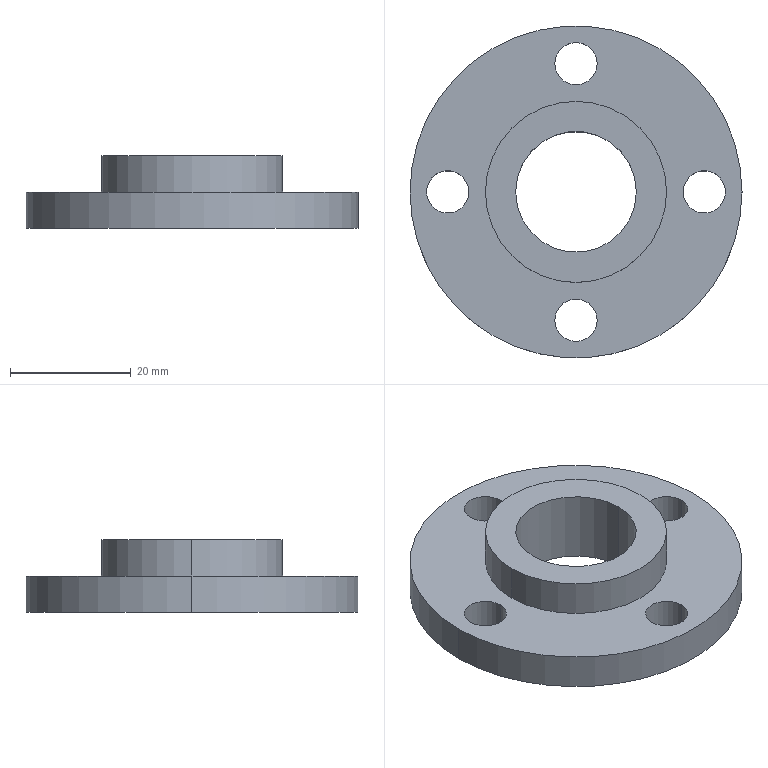Part | STEP file | BCC3 H16_9 | 1 solid | 17 faces | box 55 x 55 x 12 mm | volume 13803 mm3 | cylinder 14 | plane 3 | commonest cylinder face diameters 7 x8 20 x2 30 x2 55 x2
STEP:
#1=CARTESIAN_POINT('',(0.,0.,0.));
#2=DIRECTION('',(0.,0.,1.));
#3=DIRECTION('',(1.,0.,0.));
#4=AXIS2_PLACEMENT_3D('',#1,#2,#3);
#5=CARTESIAN_POINT('',(-17.75,0.,0.));
#6=VERTEX_POINT('',#5);
#7=CARTESIAN_POINT('',(-17.75,0.,6.));
#8=VERTEX_POINT('',#7);
#9=CARTESIAN_POINT('',(-17.75,0.,0.));
#10=DIRECTION('',(0.,0.,1.));
#11=VECTOR('',#10,1.);
#12=LINE('',#9,#11);
#13=CARTESIAN_POINT('',(-21.25,0.,0.));
#14=DIRECTION('',(0.,0.,1.));
#15=DIRECTION('',(1.,0.,0.));
#16=AXIS2_PLACEMENT_3D('',#13,#14,#15);
#17=CYLINDRICAL_SURFACE('',#16,3.5);
#18=CARTESIAN_POINT('',(6.283,0.));
#19=DIRECTION('',(0.,1.));
#20=VECTOR('',#19,1.);
#21=LINE('',#18,#20);
#22=(GEOMETRIC_REPRESENTATION_CONTEXT(2)PARAMETRIC_REPRESENTATION_CONTEXT()REPRESENTATION_CONTEXT('',''));
#23=DEFINITIONAL_REPRESENTATION('',(#21),#22);
#24=PCURVE('',#17,#23);
#25=CARTESIAN_POINT('',(-21.25,0.,0.));
#26=DIRECTION('',(0.,0.,1.));
#27=DIRECTION('',(1.,0.,0.));
#28=AXIS2_PLACEMENT_3D('',#25,#26,#27);
#29=CYLINDRICAL_SURFACE('',#28,3.5);
#30=CARTESIAN_POINT('',(0.,0.));
#31=DIRECTION('',(0.,1.));
#32=VECTOR('',#31,1.);
#33=LINE('',#30,#32);
#34=(GEOMETRIC_REPRESENTATION_CONTEXT(2)PARAMETRIC_REPRESENTATION_CONTEXT()REPRESENTATION_CONTEXT('',''));
#35=DEFINITIONAL_REPRESENTATION('',(#33),#34);
#36=PCURVE('',#29,#35);
#37=SURFACE_CURVE('',#12,(#24,#36),.PCURVE_S1.);
#38=EDGE_CURVE('',#6,#8,#37,.T.);
#39=ORIENTED_EDGE('',*,*,#38,.T.);
#40=CARTESIAN_POINT('',(-24.75,0.,6.));
#41=VERTEX_POINT('',#40);
#42=CARTESIAN_POINT('',(-21.25,0.,6.));
#43=DIRECTION('',(0.,0.,1.));
#44=DIRECTION('',(0.,1.,0.));
#45=AXIS2_PLACEMENT_3D('',#42,#43,#44);
#46=CIRCLE('',#45,3.5);
#47=CARTESIAN_POINT('',(1.571,6.));
#48=DIRECTION('',(1.,0.));
#49=VECTOR('',#48,1.);
#50=LINE('',#47,#49);
#51=(GEOMETRIC_REPRESENTATION_CONTEXT(2)PARAMETRIC_REPRESENTATION_CONTEXT()REPRESENTATION_CONTEXT('',''));
#52=DEFINITIONAL_REPRESENTATION('',(#50),#51);
#53=PCURVE('',#17,#52);
#54=CARTESIAN_POINT('',(0.,0.,6.));
#55=DIRECTION('',(0.,0.,1.));
#56=DIRECTION('',(1.,0.,0.));
#57=AXIS2_PLACEMENT_3D('',#54,#55,#56);
#58=PLANE('',#57);
#59=CARTESIAN_POINT('',(-21.25,0.));
#60=DIRECTION('',(0.,1.));
#61=AXIS2_PLACEMENT_2D('',#59,#60);
#62=CIRCLE('',#61,3.5);
#63=(GEOMETRIC_REPRESENTATION_CONTEXT(2)PARAMETRIC_REPRESENTATION_CONTEXT()REPRESENTATION_CONTEXT('',''));
#64=DEFINITIONAL_REPRESENTATION('',(#62),#63);
#65=PCURVE('',#58,#64);
#66=SURFACE_CURVE('',#46,(#53,#65),.PCURVE_S1.);
#67=EDGE_CURVE('',#41,#8,#66,.T.);
#68=ORIENTED_EDGE('',*,*,#67,.F.);
#69=CARTESIAN_POINT('',(-24.75,0.,0.));
#70=VERTEX_POINT('',#69);
#71=CARTESIAN_POINT('',(-24.75,0.,0.));
#72=DIRECTION('',(0.,0.,1.));
#73=VECTOR('',#72,1.);
#74=LINE('',#71,#73);
#75=CARTESIAN_POINT('',(3.142,0.));
#76=DIRECTION('',(0.,1.));
#77=VECTOR('',#76,1.);
#78=LINE('',#75,#77);
#79=(GEOMETRIC_REPRESENTATION_CONTEXT(2)PARAMETRIC_REPRESENTATION_CONTEXT()REPRESENTATION_CONTEXT('',''));
#80=DEFINITIONAL_REPRESENTATION('',(#78),#79);
#81=PCURVE('',#17,#80);
#82=CARTESIAN_POINT('',(3.142,0.));
#83=DIRECTION('',(0.,1.));
#84=VECTOR('',#83,1.);
#85=LINE('',#82,#84);
#86=(GEOMETRIC_REPRESENTATION_CONTEXT(2)PARAMETRIC_REPRESENTATION_CONTEXT()REPRESENTATION_CONTEXT('',''));
#87=DEFINITIONAL_REPRESENTATION('',(#85),#86);
#88=PCURVE('',#29,#87);
#89=SURFACE_CURVE('',#74,(#81,#88),.PCURVE_S1.);
#90=EDGE_CURVE('',#70,#41,#89,.T.);
#91=ORIENTED_EDGE('',*,*,#90,.F.);
#92=CARTESIAN_POINT('',(-21.25,0.,0.));
#93=DIRECTION('',(0.,0.,1.));
#94=DIRECTION('',(0.,1.,0.));
#95=AXIS2_PLACEMENT_3D('',#92,#93,#94);
#96=CIRCLE('',#95,3.5);
#97=CARTESIAN_POINT('',(1.571,0.));
#98=DIRECTION('',(1.,0.));
#99=VECTOR('',#98,1.);
#100=LINE('',#97,#99);
#101=(GEOMETRIC_REPRESENTATION_CONTEXT(2)PARAMETRIC_REPRESENTATION_CONTEXT()REPRESENTATION_CONTEXT('',''));
#102=DEFINITIONAL_REPRESENTATION('',(#100),#101);
#103=PCURVE('',#17,#102);
#104=CARTESIAN_POINT('',(0.,0.,0.));
#105=DIRECTION('',(0.,0.,1.));
#106=DIRECTION('',(1.,0.,0.));
#107=AXIS2_PLACEMENT_3D('',#104,#105,#106);
#108=PLANE('',#107);
#109=CARTESIAN_POINT('',(-21.25,0.));
#110=DIRECTION('',(0.,1.));
#111=AXIS2_PLACEMENT_2D('',#109,#110);
#112=CIRCLE('',#111,3.5);
#113=(GEOMETRIC_REPRESENTATION_CONTEXT(2)PARAMETRIC_REPRESENTATION_CONTEXT()REPRESENTATION_CONTEXT('',''));
#114=DEFINITIONAL_REPRESENTATION('',(#112),#113);
#115=PCURVE('',#108,#114);
#116=SURFACE_CURVE('',#96,(#103,#115),.PCURVE_S1.);
#117=EDGE_CURVE('',#70,#6,#116,.T.);
#118=ORIENTED_EDGE('',*,*,#117,.T.);
#119=EDGE_LOOP('',(#39,#68,#91,#118));
#120=FACE_BOUND('',#119,.F.);
#121=ADVANCED_FACE('',(#120),#17,.F.);
#122=CARTESIAN_POINT('',(3.5,-21.25,0.));
#123=VERTEX_POINT('',#122);
#124=CARTESIAN_POINT('',(3.5,-21.25,6.));
#125=VERTEX_POINT('',#124);
#126=CARTESIAN_POINT('',(3.5,-21.25,0.));
#127=DIRECTION('',(0.,0.,1.));
#128=VECTOR('',#127,1.);
#129=LINE('',#126,#128);
#130=CARTESIAN_POINT('',(0.,-21.25,0.));
#131=DIRECTION('',(0.,0.,1.));
#132=DIRECTION('',(1.,0.,0.));
#133=AXIS2_PLACEMENT_3D('',#130,#131,#132);
#134=CYLINDRICAL_SURFACE('',#133,3.5);
#135=CARTESIAN_POINT('',(6.283,0.));
#136=DIRECTION('',(0.,1.));
#137=VECTOR('',#136,1.);
#138=LINE('',#135,#137);
#139=(GEOMETRIC_REPRESENTATION_CONTEXT(2)PARAMETRIC_REPRESENTATION_CONTEXT()REPRESENTATION_CONTEXT('',''));
#140=DEFINITIONAL_REPRESENTATION('',(#138),#139);
#141=PCURVE('',#134,#140);
#142=CARTESIAN_POINT('',(0.,-21.25,0.));
#143=DIRECTION('',(0.,0.,1.));
#144=DIRECTION('',(1.,0.,0.));
#145=AXIS2_PLACEMENT_3D('',#142,#143,#144);
#146=CYLINDRICAL_SURFACE('',#145,3.5);
#147=CARTESIAN_POINT('',(0.,0.));
#148=DIRECTION('',(0.,1.));
#149=VECTOR('',#148,1.);
#150=LINE('',#147,#149);
#151=(GEOMETRIC_REPRESENTATION_CONTEXT(2)PARAMETRIC_REPRESENTATION_CONTEXT()REPRESENTATION_CONTEXT('',''));
#152=DEFINITIONAL_REPRESENTATION('',(#150),#151);
#153=PCURVE('',#146,#152);
#154=SURFACE_CURVE('',#129,(#141,#153),.PCURVE_S1.);
#155=EDGE_CURVE('',#123,#125,#154,.T.);
#156=ORIENTED_EDGE('',*,*,#155,.T.);
#157=CARTESIAN_POINT('',(-3.5,-21.25,6.));
#158=VERTEX_POINT('',#157);
#159=CARTESIAN_POINT('',(0.,-21.25,6.));
#160=DIRECTION('',(0.,0.,1.));
#161=DIRECTION('',(-1.,0.,0.));
#162=AXIS2_PLACEMENT_3D('',#159,#160,#161);
#163=CIRCLE('',#162,3.5);
#164=CARTESIAN_POINT('',(3.142,6.));
#165=DIRECTION('',(1.,0.));
#166=VECTOR('',#165,1.);
#167=LINE('',#164,#166);
#168=(GEOMETRIC_REPRESENTATION_CONTEXT(2)PARAMETRIC_REPRESENTATION_CONTEXT()REPRESENTATION_CONTEXT('',''));
#169=DEFINITIONAL_REPRESENTATION('',(#167),#168);
#170=PCURVE('',#134,#169);
#171=CARTESIAN_POINT('',(0.,-21.25));
#172=DIRECTION('',(-1.,0.));
#173=AXIS2_PLACEMENT_2D('',#171,#172);
#174=CIRCLE('',#173,3.5);
#175=(GEOMETRIC_REPRESENTATION_CONTEXT(2)PARAMETRIC_REPRESENTATION_CONTEXT()REPRESENTATION_CONTEXT('',''));
#176=DEFINITIONAL_REPRESENTATION('',(#174),#175);
#177=PCURVE('',#58,#176);
#178=SURFACE_CURVE('',#163,(#170,#177),.PCURVE_S1.);
#179=EDGE_CURVE('',#158,#125,#178,.T.);
#180=ORIENTED_EDGE('',*,*,#179,.F.);
#181=CARTESIAN_POINT('',(-3.5,-21.25,0.));
#182=VERTEX_POINT('',#181);
#183=CARTESIAN_POINT('',(-3.5,-21.25,0.));
#184=DIRECTION('',(0.,0.,1.));
#185=VECTOR('',#184,1.);
#186=LINE('',#183,#185);
#187=CARTESIAN_POINT('',(3.142,0.));
#188=DIRECTION('',(0.,1.));
#189=VECTOR('',#188,1.);
#190=LINE('',#187,#189);
#191=(GEOMETRIC_REPRESENTATION_CONTEXT(2)PARAMETRIC_REPRESENTATION_CONTEXT()REPRESENTATION_CONTEXT('',''));
#192=DEFINITIONAL_REPRESENTATION('',(#190),#191);
#193=PCURVE('',#134,#192);
#194=CARTESIAN_POINT('',(3.142,0.));
#195=DIRECTION('',(0.,1.));
#196=VECTOR('',#195,1.);
#197=LINE('',#194,#196);
#198=(GEOMETRIC_REPRESENTATION_CONTEXT(2)PARAMETRIC_REPRESENTATION_CONTEXT()REPRESENTATION_CONTEXT('',''));
#199=DEFINITIONAL_REPRESENTATION('',(#197),#198);
#200=PCURVE('',#146,#199);
#201=SURFACE_CURVE('',#186,(#193,#200),.PCURVE_S1.);
#202=EDGE_CURVE('',#182,#158,#201,.T.);
#203=ORIENTED_EDGE('',*,*,#202,.F.);
#204=CARTESIAN_POINT('',(0.,-21.25,0.));
#205=DIRECTION('',(0.,0.,1.));
#206=DIRECTION('',(-1.,0.,0.));
#207=AXIS2_PLACEMENT_3D('',#204,#205,#206);
#208=CIRCLE('',#207,3.5);
#209=CARTESIAN_POINT('',(3.142,0.));
#210=DIRECTION('',(1.,0.));
#211=VECTOR('',#210,1.);
#212=LINE('',#209,#211);
#213=(GEOMETRIC_REPRESENTATION_CONTEXT(2)PARAMETRIC_REPRESENTATION_CONTEXT()REPRESENTATION_CONTEXT('',''));
#214=DEFINITIONAL_REPRESENTATION('',(#212),#213);
#215=PCURVE('',#134,#214);
#216=CARTESIAN_POINT('',(0.,-21.25));
#217=DIRECTION('',(-1.,0.));
#218=AXIS2_PLACEMENT_2D('',#216,#217);
#219=CIRCLE('',#218,3.5);
#220=(GEOMETRIC_REPRESENTATION_CONTEXT(2)PARAMETRIC_REPRESENTATION_CONTEXT()REPRESENTATION_CONTEXT('',''));
#221=DEFINITIONAL_REPRESENTATION('',(#219),#220);
#222=PCURVE('',#108,#221);
#223=SURFACE_CURVE('',#208,(#215,#222),.PCURVE_S1.);
#224=EDGE_CURVE('',#182,#123,#223,.T.);
#225=ORIENTED_EDGE('',*,*,#224,.T.);
#226=EDGE_LOOP('',(#156,#180,#203,#225));
#227=FACE_BOUND('',#226,.F.);
#228=ADVANCED_FACE('',(#227),#134,.F.);
#229=CARTESIAN_POINT('',(24.75,0.,0.));
#230=VERTEX_POINT('',#229);
#231=CARTESIAN_POINT('',(24.75,0.,6.));
#232=VERTEX_POINT('',#231);
#233=CARTESIAN_POINT('',(24.75,0.,0.));
#234=DIRECTION('',(0.,0.,1.));
#235=VECTOR('',#234,1.);
#236=LINE('',#233,#235);
#237=CARTESIAN_POINT('',(21.25,0.,0.));
#238=DIRECTION('',(0.,0.,1.));
#239=DIRECTION('',(1.,0.,0.));
#240=AXIS2_PLACEMENT_3D('',#237,#238,#239);
#241=CYLINDRICAL_SURFACE('',#240,3.5);
#242=CARTESIAN_POINT('',(6.283,0.));
#243=DIRECTION('',(0.,1.));
#244=VECTOR('',#243,1.);
#245=LINE('',#242,#244);
#246=(GEOMETRIC_REPRESENTATION_CONTEXT(2)PARAMETRIC_REPRESENTATION_CONTEXT()REPRESENTATION_CONTEXT('',''));
#247=DEFINITIONAL_REPRESENTATION('',(#245),#246);
#248=PCURVE('',#241,#247);
#249=CARTESIAN_POINT('',(21.25,0.,0.));
#250=DIRECTION('',(0.,0.,1.));
#251=DIRECTION('',(1.,0.,0.));
#252=AXIS2_PLACEMENT_3D('',#249,#250,#251);
#253=CYLINDRICAL_SURFACE('',#252,3.5);
#254=CARTESIAN_POINT('',(0.,0.));
#255=DIRECTION('',(0.,1.));
#256=VECTOR('',#255,1.);
#257=LINE('',#254,#256);
#258=(GEOMETRIC_REPRESENTATION_CONTEXT(2)PARAMETRIC_REPRESENTATION_CONTEXT()REPRESENTATION_CONTEXT('',''));
#259=DEFINITIONAL_REPRESENTATION('',(#257),#258);
#260=PCURVE('',#253,#259);
#261=SURFACE_CURVE('',#236,(#248,#260),.PCURVE_S1.);
#262=EDGE_CURVE('',#230,#232,#261,.T.);
#263=ORIENTED_EDGE('',*,*,#262,.T.);
#264=CARTESIAN_POINT('',(17.75,0.,6.));
#265=VERTEX_POINT('',#264);
#266=CARTESIAN_POINT('',(21.25,0.,6.));
#267=DIRECTION('',(0.,0.,1.));
#268=DIRECTION('',(0.,-1.,0.));
#269=AXIS2_PLACEMENT_3D('',#266,#267,#268);
#270=CIRCLE('',#269,3.5);
#271=CARTESIAN_POINT('',(-1.571,6.));
#272=DIRECTION('',(1.,0.));
#273=VECTOR('',#272,1.);
#274=LINE('',#271,#273);
#275=(GEOMETRIC_REPRESENTATION_CONTEXT(2)PARAMETRIC_REPRESENTATION_CONTEXT()REPRESENTATION_CONTEXT('',''));
#276=DEFINITIONAL_REPRESENTATION('',(#274),#275);
#277=PCURVE('',#241,#276);
#278=CARTESIAN_POINT('',(21.25,0.));
#279=DIRECTION('',(0.,-1.));
#280=AXIS2_PLACEMENT_2D('',#278,#279);
#281=CIRCLE('',#280,3.5);
#282=(GEOMETRIC_REPRESENTATION_CONTEXT(2)PARAMETRIC_REPRESENTATION_CONTEXT()REPRESENTATION_CONTEXT('',''));
#283=DEFINITIONAL_REPRESENTATION('',(#281),#282);
#284=PCURVE('',#58,#283);
#285=SURFACE_CURVE('',#270,(#277,#284),.PCURVE_S1.);
#286=EDGE_CURVE('',#265,#232,#285,.T.);
#287=ORIENTED_EDGE('',*,*,#286,.F.);
#288=CARTESIAN_POINT('',(17.75,0.,0.));
#289=VERTEX_POINT('',#288);
#290=CARTESIAN_POINT('',(17.75,0.,0.));
#291=DIRECTION('',(0.,0.,1.));
#292=VECTOR('',#291,1.);
#293=LINE('',#290,#292);
#294=CARTESIAN_POINT('',(3.142,0.));
#295=DIRECTION('',(0.,1.));
#296=VECTOR('',#295,1.);
#297=LINE('',#294,#296);
#298=(GEOMETRIC_REPRESENTATION_CONTEXT(2)PARAMETRIC_REPRESENTATION_CONTEXT()REPRESENTATION_CONTEXT('',''));
#299=DEFINITIONAL_REPRESENTATION('',(#297),#298);
#300=PCURVE('',#241,#299);
#301=CARTESIAN_POINT('',(3.142,0.));
#302=DIRECTION('',(0.,1.));
#303=VECTOR('',#302,1.);
#304=LINE('',#301,#303);
#305=(GEOMETRIC_REPRESENTATION_CONTEXT(2)PARAMETRIC_REPRESENTATION_CONTEXT()REPRESENTATION_CONTEXT('',''));
#306=DEFINITIONAL_REPRESENTATION('',(#304),#305);
#307=PCURVE('',#253,#306);
#308=SURFACE_CURVE('',#293,(#300,#307),.PCURVE_S1.);
#309=EDGE_CURVE('',#289,#265,#308,.T.);
#310=ORIENTED_EDGE('',*,*,#309,.F.);
#311=CARTESIAN_POINT('',(21.25,0.,0.));
#312=DIRECTION('',(0.,0.,1.));
#313=DIRECTION('',(0.,-1.,0.));
#314=AXIS2_PLACEMENT_3D('',#311,#312,#313);
#315=CIRCLE('',#314,3.5);
#316=CARTESIAN_POINT('',(-1.571,0.));
#317=DIRECTION('',(1.,0.));
#318=VECTOR('',#317,1.);
#319=LINE('',#316,#318);
#320=(GEOMETRIC_REPRESENTATION_CONTEXT(2)PARAMETRIC_REPRESENTATION_CONTEXT()REPRESENTATION_CONTEXT('',''));
#321=DEFINITIONAL_REPRESENTATION('',(#319),#320);
#322=PCURVE('',#241,#321);
#323=CARTESIAN_POINT('',(21.25,0.));
#324=DIRECTION('',(0.,-1.));
#325=AXIS2_PLACEMENT_2D('',#323,#324);
#326=CIRCLE('',#325,3.5);
#327=(GEOMETRIC_REPRESENTATION_CONTEXT(2)PARAMETRIC_REPRESENTATION_CONTEXT()REPRESENTATION_CONTEXT('',''));
#328=DEFINITIONAL_REPRESENTATION('',(#326),#327);
#329=PCURVE('',#108,#328);
#330=SURFACE_CURVE('',#315,(#322,#329),.PCURVE_S1.);
#331=EDGE_CURVE('',#289,#230,#330,.T.);
#332=ORIENTED_EDGE('',*,*,#331,.T.);
#333=EDGE_LOOP('',(#263,#287,#310,#332));
#334=FACE_BOUND('',#333,.F.);
#335=ADVANCED_FACE('',(#334),#241,.F.);
#336=CARTESIAN_POINT('',(3.5,21.25,0.));
#337=VERTEX_POINT('',#336);
#338=CARTESIAN_POINT('',(3.5,21.25,6.));
#339=VERTEX_POINT('',#338);
#340=CARTESIAN_POINT('',(3.5,21.25,0.));
#341=DIRECTION('',(0.,0.,1.));
#342=VECTOR('',#341,1.);
#343=LINE('',#340,#342);
#344=CARTESIAN_POINT('',(0.,21.25,0.));
#345=DIRECTION('',(0.,0.,1.));
#346=DIRECTION('',(1.,0.,0.));
#347=AXIS2_PLACEMENT_3D('',#344,#345,#346);
#348=CYLINDRICAL_SURFACE('',#347,3.5);
#349=CARTESIAN_POINT('',(6.283,0.));
#350=DIRECTION('',(0.,1.));
#351=VECTOR('',#350,1.);
#352=LINE('',#349,#351);
#353=(GEOMETRIC_REPRESENTATION_CONTEXT(2)PARAMETRIC_REPRESENTATION_CONTEXT()REPRESENTATION_CONTEXT('',''));
#354=DEFINITIONAL_REPRESENTATION('',(#352),#353);
#355=PCURVE('',#348,#354);
#356=CARTESIAN_POINT('',(0.,21.25,0.));
#357=DIRECTION('',(0.,0.,1.));
#358=DIRECTION('',(1.,0.,0.));
#359=AXIS2_PLACEMENT_3D('',#356,#357,#358);
#360=CYLINDRICAL_SURFACE('',#359,3.5);
#361=CARTESIAN_POINT('',(0.,0.));
#362=DIRECTION('',(0.,1.));
#363=VECTOR('',#362,1.);
#364=LINE('',#361,#363);
#365=(GEOMETRIC_REPRESENTATION_CONTEXT(2)PARAMETRIC_REPRESENTATION_CONTEXT()REPRESENTATION_CONTEXT('',''));
#366=DEFINITIONAL_REPRESENTATION('',(#364),#365);
#367=PCURVE('',#360,#366);
#368=SURFACE_CURVE('',#343,(#355,#367),.PCURVE_S1.);
#369=EDGE_CURVE('',#337,#339,#368,.T.);
#370=ORIENTED_EDGE('',*,*,#369,.T.);
#371=CARTESIAN_POINT('',(-3.5,21.25,6.));
#372=VERTEX_POINT('',#371);
#373=CARTESIAN_POINT('',(0.,21.25,6.));
#374=DIRECTION('',(0.,0.,1.));
#375=DIRECTION('',(1.,0.,0.));
#376=AXIS2_PLACEMENT_3D('',#373,#374,#375);
#377=CIRCLE('',#376,3.5);
#378=CARTESIAN_POINT('',(0.,6.));
#379=DIRECTION('',(1.,0.));
#380=VECTOR('',#379,1.);
#381=LINE('',#378,#380);
#382=(GEOMETRIC_REPRESENTATION_CONTEXT(2)PARAMETRIC_REPRESENTATION_CONTEXT()REPRESENTATION_CONTEXT('',''));
#383=DEFINITIONAL_REPRESENTATION('',(#381),#382);
#384=PCURVE('',#348,#383);
#385=CARTESIAN_POINT('',(0.,21.25));
#386=DIRECTION('',(1.,0.));
#387=AXIS2_PLACEMENT_2D('',#385,#386);
#388=CIRCLE('',#387,3.5);
#389=(GEOMETRIC_REPRESENTATION_CONTEXT(2)PARAMETRIC_REPRESENTATION_CONTEXT()REPRESENTATION_CONTEXT('',''));
#390=DEFINITIONAL_REPRESENTATION('',(#388),#389);
#391=PCURVE('',#58,#390);
#392=SURFACE_CURVE('',#377,(#384,#391),.PCURVE_S1.);
#393=EDGE_CURVE('',#372,#339,#392,.T.);
#394=ORIENTED_EDGE('',*,*,#393,.F.);
#395=CARTESIAN_POINT('',(-3.5,21.25,0.));
#396=VERTEX_POINT('',#395);
#397=CARTESIAN_POINT('',(-3.5,21.25,0.));
#398=DIRECTION('',(0.,0.,1.));
#399=VECTOR('',#398,1.);
#400=LINE('',#397,#399);
#401=CARTESIAN_POINT('',(3.142,0.));
#402=DIRECTION('',(0.,1.));
#403=VECTOR('',#402,1.);
#404=LINE('',#401,#403);
#405=(GEOMETRIC_REPRESENTATION_CONTEXT(2)PARAMETRIC_REPRESENTATION_CONTEXT()REPRESENTATION_CONTEXT('',''));
#406=DEFINITIONAL_REPRESENTATION('',(#404),#405);
#407=PCURVE('',#348,#406);
#408=CARTESIAN_POINT('',(3.142,0.));
#409=DIRECTION('',(0.,1.));
#410=VECTOR('',#409,1.);
#411=LINE('',#408,#410);
#412=(GEOMETRIC_REPRESENTATION_CONTEXT(2)PARAMETRIC_REPRESENTATION_CONTEXT()REPRESENTATION_CONTEXT('',''));
#413=DEFINITIONAL_REPRESENTATION('',(#411),#412);
#414=PCURVE('',#360,#413);
#415=SURFACE_CURVE('',#400,(#407,#414),.PCURVE_S1.);
#416=EDGE_CURVE('',#396,#372,#415,.T.);
#417=ORIENTED_EDGE('',*,*,#416,.F.);
#418=CARTESIAN_POINT('',(0.,21.25,0.));
#419=DIRECTION('',(0.,0.,1.));
#420=DIRECTION('',(1.,0.,0.));
#421=AXIS2_PLACEMENT_3D('',#418,#419,#420);
#422=CIRCLE('',#421,3.5);
#423=CARTESIAN_POINT('',(0.,0.));
#424=DIRECTION('',(1.,0.));
#425=VECTOR('',#424,1.);
#426=LINE('',#423,#425);
#427=(GEOMETRIC_REPRESENTATION_CONTEXT(2)PARAMETRIC_REPRESENTATION_CONTEXT()REPRESENTATION_CONTEXT('',''));
#428=DEFINITIONAL_REPRESENTATION('',(#426),#427);
#429=PCURVE('',#348,#428);
#430=CARTESIAN_POINT('',(0.,21.25));
#431=DIRECTION('',(1.,0.));
#432=AXIS2_PLACEMENT_2D('',#430,#431);
#433=CIRCLE('',#432,3.5);
#434=(GEOMETRIC_REPRESENTATION_CONTEXT(2)PARAMETRIC_REPRESENTATION_CONTEXT()REPRESENTATION_CONTEXT('',''));
#435=DEFINITIONAL_REPRESENTATION('',(#433),#434);
#436=PCURVE('',#108,#435);
#437=SURFACE_CURVE('',#422,(#429,#436),.PCURVE_S1.);
#438=EDGE_CURVE('',#396,#337,#437,.T.);
#439=ORIENTED_EDGE('',*,*,#438,.T.);
#440=EDGE_LOOP('',(#370,#394,#417,#439));
#441=FACE_BOUND('',#440,.F.);
#442=ADVANCED_FACE('',(#441),#348,.F.);
#443=CARTESIAN_POINT('',(15.,0.,6.));
#444=VERTEX_POINT('',#443);
#445=CARTESIAN_POINT('',(-15.,0.,6.));
#446=VERTEX_POINT('',#445);
#447=CARTESIAN_POINT('',(0.,0.,6.));
#448=DIRECTION('',(0.,0.,1.));
#449=DIRECTION('',(1.,0.,0.));
#450=AXIS2_PLACEMENT_3D('',#447,#448,#449);
#451=CIRCLE('',#450,15.);
#452=CARTESIAN_POINT('',(0.,0.,6.));
#453=DIRECTION('',(0.,0.,1.));
#454=DIRECTION('',(1.,0.,0.));
#455=AXIS2_PLACEMENT_3D('',#452,#453,#454);
#456=CYLINDRICAL_SURFACE('',#455,15.);
#457=CARTESIAN_POINT('',(0.,0.));
#458=DIRECTION('',(1.,0.));
#459=VECTOR('',#458,1.);
#460=LINE('',#457,#459);
#461=(GEOMETRIC_REPRESENTATION_CONTEXT(2)PARAMETRIC_REPRESENTATION_CONTEXT()REPRESENTATION_CONTEXT('',''));
#462=DEFINITIONAL_REPRESENTATION('',(#460),#461);
#463=PCURVE('',#456,#462);
#464=CARTESIAN_POINT('',(0.,0.));
#465=DIRECTION('',(1.,0.));
#466=AXIS2_PLACEMENT_2D('',#464,#465);
#467=CIRCLE('',#466,15.);
#468=(GEOMETRIC_REPRESENTATION_CONTEXT(2)PARAMETRIC_REPRESENTATION_CONTEXT()REPRESENTATION_CONTEXT('',''));
#469=DEFINITIONAL_REPRESENTATION('',(#467),#468);
#470=PCURVE('',#58,#469);
#471=SURFACE_CURVE('',#451,(#463,#470),.PCURVE_S1.);
#472=EDGE_CURVE('',#444,#446,#471,.T.);
#473=ORIENTED_EDGE('',*,*,#472,.T.);
#474=CARTESIAN_POINT('',(-15.,0.,12.));
#475=VERTEX_POINT('',#474);
#476=CARTESIAN_POINT('',(-15.,0.,6.));
#477=DIRECTION('',(0.,0.,1.));
#478=VECTOR('',#477,1.);
#479=LINE('',#476,#478);
#480=CARTESIAN_POINT('',(3.142,0.));
#481=DIRECTION('',(0.,1.));
#482=VECTOR('',#481,1.);
#483=LINE('',#480,#482);
#484=(GEOMETRIC_REPRESENTATION_CONTEXT(2)PARAMETRIC_REPRESENTATION_CONTEXT()REPRESENTATION_CONTEXT('',''));
#485=DEFINITIONAL_REPRESENTATION('',(#483),#484);
#486=PCURVE('',#456,#485);
#487=CARTESIAN_POINT('',(0.,0.,6.));
#488=DIRECTION('',(0.,0.,1.));
#489=DIRECTION('',(1.,0.,0.));
#490=AXIS2_PLACEMENT_3D('',#487,#488,#489);
#491=CYLINDRICAL_SURFACE('',#490,15.);
#492=CARTESIAN_POINT('',(3.142,0.));
#493=DIRECTION('',(0.,1.));
#494=VECTOR('',#493,1.);
#495=LINE('',#492,#494);
#496=(GEOMETRIC_REPRESENTATION_CONTEXT(2)PARAMETRIC_REPRESENTATION_CONTEXT()REPRESENTATION_CONTEXT('',''));
#497=DEFINITIONAL_REPRESENTATION('',(#495),#496);
#498=PCURVE('',#491,#497);
#499=SURFACE_CURVE('',#479,(#486,#498),.PCURVE_S1.);
#500=EDGE_CURVE('',#446,#475,#499,.T.);
#501=ORIENTED_EDGE('',*,*,#500,.T.);
#502=CARTESIAN_POINT('',(15.,0.,12.));
#503=VERTEX_POINT('',#502);
#504=CARTESIAN_POINT('',(0.,0.,12.));
#505=DIRECTION('',(0.,0.,1.));
#506=DIRECTION('',(1.,0.,0.));
#507=AXIS2_PLACEMENT_3D('',#504,#505,#506);
#508=CIRCLE('',#507,15.);
#509=CARTESIAN_POINT('',(0.,6.));
#510=DIRECTION('',(1.,0.));
#511=VECTOR('',#510,1.);
#512=LINE('',#509,#511);
#513=(GEOMETRIC_REPRESENTATION_CONTEXT(2)PARAMETRIC_REPRESENTATION_CONTEXT()REPRESENTATION_CONTEXT('',''));
#514=DEFINITIONAL_REPRESENTATION('',(#512),#513);
#515=PCURVE('',#456,#514);
#516=CARTESIAN_POINT('',(0.,0.,12.));
#517=DIRECTION('',(0.,0.,1.));
#518=DIRECTION('',(1.,0.,0.));
#519=AXIS2_PLACEMENT_3D('',#516,#517,#518);
#520=PLANE('',#519);
#521=CARTESIAN_POINT('',(0.,0.));
#522=DIRECTION('',(1.,0.));
#523=AXIS2_PLACEMENT_2D('',#521,#522);
#524=CIRCLE('',#523,15.);
#525=(GEOMETRIC_REPRESENTATION_CONTEXT(2)PARAMETRIC_REPRESENTATION_CONTEXT()REPRESENTATION_CONTEXT('',''));
#526=DEFINITIONAL_REPRESENTATION('',(#524),#525);
#527=PCURVE('',#520,#526);
#528=SURFACE_CURVE('',#508,(#515,#527),.PCURVE_S1.);
#529=EDGE_CURVE('',#503,#475,#528,.T.);
#530=ORIENTED_EDGE('',*,*,#529,.F.);
#531=CARTESIAN_POINT('',(15.,0.,6.));
#532=DIRECTION('',(0.,0.,1.));
#533=VECTOR('',#532,1.);
#534=LINE('',#531,#533);
#535=CARTESIAN_POINT('',(0.,0.));
#536=DIRECTION('',(0.,1.));
#537=VECTOR('',#536,1.);
#538=LINE('',#535,#537);
#539=(GEOMETRIC_REPRESENTATION_CONTEXT(2)PARAMETRIC_REPRESENTATION_CONTEXT()REPRESENTATION_CONTEXT('',''));
#540=DEFINITIONAL_REPRESENTATION('',(#538),#539);
#541=PCURVE('',#456,#540);
#542=CARTESIAN_POINT('',(6.283,0.));
#543=DIRECTION('',(0.,1.));
#544=VECTOR('',#543,1.);
#545=LINE('',#542,#544);
#546=(GEOMETRIC_REPRESENTATION_CONTEXT(2)PARAMETRIC_REPRESENTATION_CONTEXT()REPRESENTATION_CONTEXT('',''));
#547=DEFINITIONAL_REPRESENTATION('',(#545),#546);
#548=PCURVE('',#491,#547);
#549=SURFACE_CURVE('',#534,(#541,#548),.PCURVE_S1.);
#550=EDGE_CURVE('',#444,#503,#549,.T.);
#551=ORIENTED_EDGE('',*,*,#550,.F.);
#552=EDGE_LOOP('',(#473,#501,#530,#551));
#553=FACE_BOUND('',#552,.T.);
#554=ADVANCED_FACE('',(#553),#456,.T.);
#555=CARTESIAN_POINT('',(-10.,0.,12.));
#556=VERTEX_POINT('',#555);
#557=CARTESIAN_POINT('',(-10.,0.,0.));
#558=VERTEX_POINT('',#557);
#559=CARTESIAN_POINT('',(-10.,0.,12.));
#560=DIRECTION('',(0.,0.,-1.));
#561=VECTOR('',#560,1.);
#562=LINE('',#559,#561);
#563=CARTESIAN_POINT('',(0.,0.,12.));
#564=DIRECTION('',(0.,0.,-1.));
#565=DIRECTION('',(-1.,0.,0.));
#566=AXIS2_PLACEMENT_3D('',#563,#564,#565);
#567=CYLINDRICAL_SURFACE('',#566,10.);
#568=CARTESIAN_POINT('',(6.283,0.));
#569=DIRECTION('',(0.,1.));
#570=VECTOR('',#569,1.);
#571=LINE('',#568,#570);
#572=(GEOMETRIC_REPRESENTATION_CONTEXT(2)PARAMETRIC_REPRESENTATION_CONTEXT()REPRESENTATION_CONTEXT('',''));
#573=DEFINITIONAL_REPRESENTATION('',(#571),#572);
#574=PCURVE('',#567,#573);
#575=CARTESIAN_POINT('',(0.,0.,12.));
#576=DIRECTION('',(0.,0.,-1.));
#577=DIRECTION('',(-1.,0.,0.));
#578=AXIS2_PLACEMENT_3D('',#575,#576,#577);
#579=CYLINDRICAL_SURFACE('',#578,10.);
#580=CARTESIAN_POINT('',(0.,0.));
#581=DIRECTION('',(0.,1.));
#582=VECTOR('',#581,1.);
#583=LINE('',#580,#582);
#584=(GEOMETRIC_REPRESENTATION_CONTEXT(2)PARAMETRIC_REPRESENTATION_CONTEXT()REPRESENTATION_CONTEXT('',''));
#585=DEFINITIONAL_REPRESENTATION('',(#583),#584);
#586=PCURVE('',#579,#585);
#587=SURFACE_CURVE('',#562,(#574,#586),.PCURVE_S1.);
#588=EDGE_CURVE('',#556,#558,#587,.T.);
#589=ORIENTED_EDGE('',*,*,#588,.T.);
#590=CARTESIAN_POINT('',(10.,0.,0.));
#591=VERTEX_POINT('',#590);
#592=CARTESIAN_POINT('',(0.,0.,0.));
#593=DIRECTION('',(0.,0.,1.));
#594=DIRECTION('',(1.,0.,0.));
#595=AXIS2_PLACEMENT_3D('',#592,#593,#594);
#596=CIRCLE('',#595,10.);
#597=CARTESIAN_POINT('',(9.425,12.));
#598=DIRECTION('',(-1.,0.));
#599=VECTOR('',#598,1.);
#600=LINE('',#597,#599);
#601=(GEOMETRIC_REPRESENTATION_CONTEXT(2)PARAMETRIC_REPRESENTATION_CONTEXT()REPRESENTATION_CONTEXT('',''));
#602=DEFINITIONAL_REPRESENTATION('',(#600),#601);
#603=PCURVE('',#567,#602);
#604=CARTESIAN_POINT('',(0.,0.));
#605=DIRECTION('',(1.,0.));
#606=AXIS2_PLACEMENT_2D('',#604,#605);
#607=CIRCLE('',#606,10.);
#608=(GEOMETRIC_REPRESENTATION_CONTEXT(2)PARAMETRIC_REPRESENTATION_CONTEXT()REPRESENTATION_CONTEXT('',''));
#609=DEFINITIONAL_REPRESENTATION('',(#607),#608);
#610=PCURVE('',#108,#609);
#611=SURFACE_CURVE('',#596,(#603,#610),.PCURVE_S1.);
#612=EDGE_CURVE('',#558,#591,#611,.T.);
#613=ORIENTED_EDGE('',*,*,#612,.T.);
#614=CARTESIAN_POINT('',(10.,0.,12.));
#615=VERTEX_POINT('',#614);
#616=CARTESIAN_POINT('',(10.,0.,12.));
#617=DIRECTION('',(0.,0.,-1.));
#618=VECTOR('',#617,1.);
#619=LINE('',#616,#618);
#620=CARTESIAN_POINT('',(3.142,0.));
#621=DIRECTION('',(0.,1.));
#622=VECTOR('',#621,1.);
#623=LINE('',#620,#622);
#624=(GEOMETRIC_REPRESENTATION_CONTEXT(2)PARAMETRIC_REPRESENTATION_CONTEXT()REPRESENTATION_CONTEXT('',''));
#625=DEFINITIONAL_REPRESENTATION('',(#623),#624);
#626=PCURVE('',#567,#625);
#627=CARTESIAN_POINT('',(3.142,0.));
#628=DIRECTION('',(0.,1.));
#629=VECTOR('',#628,1.);
#630=LINE('',#627,#629);
#631=(GEOMETRIC_REPRESENTATION_CONTEXT(2)PARAMETRIC_REPRESENTATION_CONTEXT()REPRESENTATION_CONTEXT('',''));
#632=DEFINITIONAL_REPRESENTATION('',(#630),#631);
#633=PCURVE('',#579,#632);
#634=SURFACE_CURVE('',#619,(#626,#633),.PCURVE_S1.);
#635=EDGE_CURVE('',#615,#591,#634,.T.);
#636=ORIENTED_EDGE('',*,*,#635,.F.);
#637=CARTESIAN_POINT('',(0.,0.,12.));
#638=DIRECTION('',(0.,0.,1.));
#639=DIRECTION('',(1.,0.,0.));
#640=AXIS2_PLACEMENT_3D('',#637,#638,#639);
#641=CIRCLE('',#640,10.);
#642=CARTESIAN_POINT('',(9.425,0.));
#643=DIRECTION('',(-1.,0.));
#644=VECTOR('',#643,1.);
#645=LINE('',#642,#644);
#646=(GEOMETRIC_REPRESENTATION_CONTEXT(2)PARAMETRIC_REPRESENTATION_CONTEXT()REPRESENTATION_CONTEXT('',''));
#647=DEFINITIONAL_REPRESENTATION('',(#645),#646);
#648=PCURVE('',#567,#647);
#649=CARTESIAN_POINT('',(0.,0.));
#650=DIRECTION('',(1.,0.));
#651=AXIS2_PLACEMENT_2D('',#649,#650);
#652=CIRCLE('',#651,10.);
#653=(GEOMETRIC_REPRESENTATION_CONTEXT(2)PARAMETRIC_REPRESENTATION_CONTEXT()REPRESENTATION_CONTEXT('',''));
#654=DEFINITIONAL_REPRESENTATION('',(#652),#653);
#655=PCURVE('',#520,#654);
#656=SURFACE_CURVE('',#641,(#648,#655),.PCURVE_S1.);
#657=EDGE_CURVE('',#556,#615,#656,.T.);
#658=ORIENTED_EDGE('',*,*,#657,.F.);
#659=EDGE_LOOP('',(#589,#613,#636,#658));
#660=FACE_BOUND('',#659,.F.);
#661=ADVANCED_FACE('',(#660),#567,.F.);
#662=CARTESIAN_POINT('',(27.5,0.,6.));
#663=VERTEX_POINT('',#662);
#664=CARTESIAN_POINT('',(-27.5,0.,6.));
#665=VERTEX_POINT('',#664);
#666=CARTESIAN_POINT('',(0.,0.,6.));
#667=DIRECTION('',(0.,0.,1.));
#668=DIRECTION('',(1.,0.,0.));
#669=AXIS2_PLACEMENT_3D('',#666,#667,#668);
#670=CIRCLE('',#669,27.5);
#671=CARTESIAN_POINT('',(0.,0.,12.));
#672=DIRECTION('',(0.,0.,-1.));
#673=DIRECTION('',(-1.,0.,0.));
#674=AXIS2_PLACEMENT_3D('',#671,#672,#673);
#675=CYLINDRICAL_SURFACE('',#674,27.5);
#676=CARTESIAN_POINT('',(3.142,6.));
#677=DIRECTION('',(-1.,0.));
#678=VECTOR('',#677,1.);
#679=LINE('',#676,#678);
#680=(GEOMETRIC_REPRESENTATION_CONTEXT(2)PARAMETRIC_REPRESENTATION_CONTEXT()REPRESENTATION_CONTEXT('',''));
#681=DEFINITIONAL_REPRESENTATION('',(#679),#680);
#682=PCURVE('',#675,#681);
#683=CARTESIAN_POINT('',(0.,0.));
#684=DIRECTION('',(1.,0.));
#685=AXIS2_PLACEMENT_2D('',#683,#684);
#686=CIRCLE('',#685,27.5);
#687=(GEOMETRIC_REPRESENTATION_CONTEXT(2)PARAMETRIC_REPRESENTATION_CONTEXT()REPRESENTATION_CONTEXT('',''));
#688=DEFINITIONAL_REPRESENTATION('',(#686),#687);
#689=PCURVE('',#58,#688);
#690=SURFACE_CURVE('',#670,(#682,#689),.PCURVE_S1.);
#691=EDGE_CURVE('',#663,#665,#690,.T.);
#692=ORIENTED_EDGE('',*,*,#691,.F.);
#693=CARTESIAN_POINT('',(27.5,0.,0.));
#694=VERTEX_POINT('',#693);
#695=CARTESIAN_POINT('',(27.5,0.,12.));
#696=DIRECTION('',(0.,0.,-1.));
#697=VECTOR('',#696,1.);
#698=LINE('',#695,#697);
#699=CARTESIAN_POINT('',(3.142,0.));
#700=DIRECTION('',(0.,1.));
#701=VECTOR('',#700,1.);
#702=LINE('',#699,#701);
#703=(GEOMETRIC_REPRESENTATION_CONTEXT(2)PARAMETRIC_REPRESENTATION_CONTEXT()REPRESENTATION_CONTEXT('',''));
#704=DEFINITIONAL_REPRESENTATION('',(#702),#703);
#705=PCURVE('',#675,#704);
#706=CARTESIAN_POINT('',(0.,0.,12.));
#707=DIRECTION('',(0.,0.,-1.));
#708=DIRECTION('',(-1.,0.,0.));
#709=AXIS2_PLACEMENT_3D('',#706,#707,#708);
#710=CYLINDRICAL_SURFACE('',#709,27.5);
#711=CARTESIAN_POINT('',(3.142,0.));
#712=DIRECTION('',(0.,1.));
#713=VECTOR('',#712,1.);
#714=LINE('',#711,#713);
#715=(GEOMETRIC_REPRESENTATION_CONTEXT(2)PARAMETRIC_REPRESENTATION_CONTEXT()REPRESENTATION_CONTEXT('',''));
#716=DEFINITIONAL_REPRESENTATION('',(#714),#715);
#717=PCURVE('',#710,#716);
#718=SURFACE_CURVE('',#698,(#705,#717),.PCURVE_S1.);
#719=EDGE_CURVE('',#663,#694,#718,.T.);
#720=ORIENTED_EDGE('',*,*,#719,.T.);
#721=CARTESIAN_POINT('',(-27.5,0.,0.));
#722=VERTEX_POINT('',#721);
#723=CARTESIAN_POINT('',(0.,0.,0.));
#724=DIRECTION('',(0.,0.,1.));
#725=DIRECTION('',(1.,0.,0.));
#726=AXIS2_PLACEMENT_3D('',#723,#724,#725);
#727=CIRCLE('',#726,27.5);
#728=CARTESIAN_POINT('',(3.142,12.));
#729=DIRECTION('',(-1.,0.));
#730=VECTOR('',#729,1.);
#731=LINE('',#728,#730);
#732=(GEOMETRIC_REPRESENTATION_CONTEXT(2)PARAMETRIC_REPRESENTATION_CONTEXT()REPRESENTATION_CONTEXT('',''));
#733=DEFINITIONAL_REPRESENTATION('',(#731),#732);
#734=PCURVE('',#675,#733);
#735=CARTESIAN_POINT('',(0.,0.));
#736=DIRECTION('',(1.,0.));
#737=AXIS2_PLACEMENT_2D('',#735,#736);
#738=CIRCLE('',#737,27.5);
#739=(GEOMETRIC_REPRESENTATION_CONTEXT(2)PARAMETRIC_REPRESENTATION_CONTEXT()REPRESENTATION_CONTEXT('',''));
#740=DEFINITIONAL_REPRESENTATION('',(#738),#739);
#741=PCURVE('',#108,#740);
#742=SURFACE_CURVE('',#727,(#734,#741),.PCURVE_S1.);
#743=EDGE_CURVE('',#694,#722,#742,.T.);
#744=ORIENTED_EDGE('',*,*,#743,.T.);
#745=CARTESIAN_POINT('',(-27.5,0.,12.));
#746=DIRECTION('',(0.,0.,-1.));
#747=VECTOR('',#746,1.);
#748=LINE('',#745,#747);
#749=CARTESIAN_POINT('',(0.,0.));
#750=DIRECTION('',(0.,1.));
#751=VECTOR('',#750,1.);
#752=LINE('',#749,#751);
#753=(GEOMETRIC_REPRESENTATION_CONTEXT(2)PARAMETRIC_REPRESENTATION_CONTEXT()REPRESENTATION_CONTEXT('',''));
#754=DEFINITIONAL_REPRESENTATION('',(#752),#753);
#755=PCURVE('',#675,#754);
#756=CARTESIAN_POINT('',(6.283,0.));
#757=DIRECTION('',(0.,1.));
#758=VECTOR('',#757,1.);
#759=LINE('',#756,#758);
#760=(GEOMETRIC_REPRESENTATION_CONTEXT(2)PARAMETRIC_REPRESENTATION_CONTEXT()REPRESENTATION_CONTEXT('',''));
#761=DEFINITIONAL_REPRESENTATION('',(#759),#760);
#762=PCURVE('',#710,#761);
#763=SURFACE_CURVE('',#748,(#755,#762),.PCURVE_S1.);
#764=EDGE_CURVE('',#665,#722,#763,.T.);
#765=ORIENTED_EDGE('',*,*,#764,.F.);
#766=EDGE_LOOP('',(#692,#720,#744,#765));
#767=FACE_BOUND('',#766,.T.);
#768=ADVANCED_FACE('',(#767),#675,.T.);
#769=ORIENTED_EDGE('',*,*,#657,.F.);
#770=CARTESIAN_POINT('',(0.,0.,12.));
#771=DIRECTION('',(0.,0.,1.));
#772=DIRECTION('',(1.,0.,0.));
#773=AXIS2_PLACEMENT_3D('',#770,#771,#772);
#774=CIRCLE('',#773,10.);
#775=CARTESIAN_POINT('',(0.,0.));
#776=DIRECTION('',(1.,0.));
#777=AXIS2_PLACEMENT_2D('',#775,#776);
#778=CIRCLE('',#777,10.);
#779=(GEOMETRIC_REPRESENTATION_CONTEXT(2)PARAMETRIC_REPRESENTATION_CONTEXT()REPRESENTATION_CONTEXT('',''));
#780=DEFINITIONAL_REPRESENTATION('',(#778),#779);
#781=PCURVE('',#520,#780);
#782=CARTESIAN_POINT('',(3.142,0.));
#783=DIRECTION('',(-1.,0.));
#784=VECTOR('',#783,1.);
#785=LINE('',#782,#784);
#786=(GEOMETRIC_REPRESENTATION_CONTEXT(2)PARAMETRIC_REPRESENTATION_CONTEXT()REPRESENTATION_CONTEXT('',''));
#787=DEFINITIONAL_REPRESENTATION('',(#785),#786);
#788=PCURVE('',#579,#787);
#789=SURFACE_CURVE('',#774,(#781,#788),.PCURVE_S1.);
#790=EDGE_CURVE('',#615,#556,#789,.T.);
#791=ORIENTED_EDGE('',*,*,#790,.F.);
#792=EDGE_LOOP('',(#769,#791));
#793=FACE_BOUND('',#792,.T.);
#794=ORIENTED_EDGE('',*,*,#529,.T.);
#795=CARTESIAN_POINT('',(0.,0.,12.));
#796=DIRECTION('',(0.,0.,1.));
#797=DIRECTION('',(1.,0.,0.));
#798=AXIS2_PLACEMENT_3D('',#795,#796,#797);
#799=CIRCLE('',#798,15.);
#800=CARTESIAN_POINT('',(0.,0.));
#801=DIRECTION('',(1.,0.));
#802=AXIS2_PLACEMENT_2D('',#800,#801);
#803=CIRCLE('',#802,15.);
#804=(GEOMETRIC_REPRESENTATION_CONTEXT(2)PARAMETRIC_REPRESENTATION_CONTEXT()REPRESENTATION_CONTEXT('',''));
#805=DEFINITIONAL_REPRESENTATION('',(#803),#804);
#806=PCURVE('',#520,#805);
#807=CARTESIAN_POINT('',(0.,6.));
#808=DIRECTION('',(1.,0.));
#809=VECTOR('',#808,1.);
#810=LINE('',#807,#809);
#811=(GEOMETRIC_REPRESENTATION_CONTEXT(2)PARAMETRIC_REPRESENTATION_CONTEXT()REPRESENTATION_CONTEXT('',''));
#812=DEFINITIONAL_REPRESENTATION('',(#810),#811);
#813=PCURVE('',#491,#812);
#814=SURFACE_CURVE('',#799,(#806,#813),.PCURVE_S1.);
#815=EDGE_CURVE('',#475,#503,#814,.T.);
#816=ORIENTED_EDGE('',*,*,#815,.T.);
#817=EDGE_LOOP('',(#794,#816));
#818=FACE_BOUND('',#817,.T.);
#819=ADVANCED_FACE('',(#793,#818),#520,.T.);
#820=ORIENTED_EDGE('',*,*,#719,.F.);
#821=CARTESIAN_POINT('',(0.,0.,6.));
#822=DIRECTION('',(0.,0.,1.));
#823=DIRECTION('',(1.,0.,0.));
#824=AXIS2_PLACEMENT_3D('',#821,#822,#823);
#825=CIRCLE('',#824,27.5);
#826=CARTESIAN_POINT('',(9.425,6.));
#827=DIRECTION('',(-1.,0.));
#828=VECTOR('',#827,1.);
#829=LINE('',#826,#828);
#830=(GEOMETRIC_REPRESENTATION_CONTEXT(2)PARAMETRIC_REPRESENTATION_CONTEXT()REPRESENTATION_CONTEXT('',''));
#831=DEFINITIONAL_REPRESENTATION('',(#829),#830);
#832=PCURVE('',#710,#831);
#833=CARTESIAN_POINT('',(0.,0.));
#834=DIRECTION('',(1.,0.));
#835=AXIS2_PLACEMENT_2D('',#833,#834);
#836=CIRCLE('',#835,27.5);
#837=(GEOMETRIC_REPRESENTATION_CONTEXT(2)PARAMETRIC_REPRESENTATION_CONTEXT()REPRESENTATION_CONTEXT('',''));
#838=DEFINITIONAL_REPRESENTATION('',(#836),#837);
#839=PCURVE('',#58,#838);
#840=SURFACE_CURVE('',#825,(#832,#839),.PCURVE_S1.);
#841=EDGE_CURVE('',#665,#663,#840,.T.);
#842=ORIENTED_EDGE('',*,*,#841,.F.);
#843=ORIENTED_EDGE('',*,*,#764,.T.);
#844=CARTESIAN_POINT('',(0.,0.,0.));
#845=DIRECTION('',(0.,0.,1.));
#846=DIRECTION('',(1.,0.,0.));
#847=AXIS2_PLACEMENT_3D('',#844,#845,#846);
#848=CIRCLE('',#847,27.5);
#849=CARTESIAN_POINT('',(9.425,12.));
#850=DIRECTION('',(-1.,0.));
#851=VECTOR('',#850,1.);
#852=LINE('',#849,#851);
#853=(GEOMETRIC_REPRESENTATION_CONTEXT(2)PARAMETRIC_REPRESENTATION_CONTEXT()REPRESENTATION_CONTEXT('',''));
#854=DEFINITIONAL_REPRESENTATION('',(#852),#853);
#855=PCURVE('',#710,#854);
#856=CARTESIAN_POINT('',(0.,0.));
#857=DIRECTION('',(1.,0.));
#858=AXIS2_PLACEMENT_2D('',#856,#857);
#859=CIRCLE('',#858,27.5);
#860=(GEOMETRIC_REPRESENTATION_CONTEXT(2)PARAMETRIC_REPRESENTATION_CONTEXT()REPRESENTATION_CONTEXT('',''));
#861=DEFINITIONAL_REPRESENTATION('',(#859),#860);
#862=PCURVE('',#108,#861);
#863=SURFACE_CURVE('',#848,(#855,#862),.PCURVE_S1.);
#864=EDGE_CURVE('',#722,#694,#863,.T.);
#865=ORIENTED_EDGE('',*,*,#864,.T.);
#866=EDGE_LOOP('',(#820,#842,#843,#865));
#867=FACE_BOUND('',#866,.T.);
#868=ADVANCED_FACE('',(#867),#710,.T.);
#869=CARTESIAN_POINT('',(-21.25,0.,0.));
#870=DIRECTION('',(0.,0.,1.));
#871=DIRECTION('',(0.,1.,0.));
#872=AXIS2_PLACEMENT_3D('',#869,#870,#871);
#873=CIRCLE('',#872,3.5);
#874=CARTESIAN_POINT('',(-21.25,0.));
#875=DIRECTION('',(0.,1.));
#876=AXIS2_PLACEMENT_2D('',#874,#875);
#877=CIRCLE('',#876,3.5);
#878=(GEOMETRIC_REPRESENTATION_CONTEXT(2)PARAMETRIC_REPRESENTATION_CONTEXT()REPRESENTATION_CONTEXT('',''));
#879=DEFINITIONAL_REPRESENTATION('',(#877),#878);
#880=PCURVE('',#108,#879);
#881=CARTESIAN_POINT('',(-4.712,0.));
#882=DIRECTION('',(1.,0.));
#883=VECTOR('',#882,1.);
#884=LINE('',#881,#883);
#885=(GEOMETRIC_REPRESENTATION_CONTEXT(2)PARAMETRIC_REPRESENTATION_CONTEXT()REPRESENTATION_CONTEXT('',''));
#886=DEFINITIONAL_REPRESENTATION('',(#884),#885);
#887=PCURVE('',#29,#886);
#888=SURFACE_CURVE('',#873,(#880,#887),.PCURVE_S1.);
#889=EDGE_CURVE('',#6,#70,#888,.T.);
#890=ORIENTED_EDGE('',*,*,#889,.T.);
#891=ORIENTED_EDGE('',*,*,#117,.T.);
#892=EDGE_LOOP('',(#890,#891));
#893=FACE_BOUND('',#892,.T.);
#894=CARTESIAN_POINT('',(0.,-21.25,0.));
#895=DIRECTION('',(0.,0.,1.));
#896=DIRECTION('',(-1.,0.,0.));
#897=AXIS2_PLACEMENT_3D('',#894,#895,#896);
#898=CIRCLE('',#897,3.5);
#899=CARTESIAN_POINT('',(0.,-21.25));
#900=DIRECTION('',(-1.,0.));
#901=AXIS2_PLACEMENT_2D('',#899,#900);
#902=CIRCLE('',#901,3.5);
#903=(GEOMETRIC_REPRESENTATION_CONTEXT(2)PARAMETRIC_REPRESENTATION_CONTEXT()REPRESENTATION_CONTEXT('',''));
#904=DEFINITIONAL_REPRESENTATION('',(#902),#903);
#905=PCURVE('',#108,#904);
#906=CARTESIAN_POINT('',(-3.142,0.));
#907=DIRECTION('',(1.,0.));
#908=VECTOR('',#907,1.);
#909=LINE('',#906,#908);
#910=(GEOMETRIC_REPRESENTATION_CONTEXT(2)PARAMETRIC_REPRESENTATION_CONTEXT()REPRESENTATION_CONTEXT('',''));
#911=DEFINITIONAL_REPRESENTATION('',(#909),#910);
#912=PCURVE('',#146,#911);
#913=SURFACE_CURVE('',#898,(#905,#912),.PCURVE_S1.);
#914=EDGE_CURVE('',#123,#182,#913,.T.);
#915=ORIENTED_EDGE('',*,*,#914,.T.);
#916=ORIENTED_EDGE('',*,*,#224,.T.);
#917=EDGE_LOOP('',(#915,#916));
#918=FACE_BOUND('',#917,.T.);
#919=CARTESIAN_POINT('',(21.25,0.,0.));
#920=DIRECTION('',(0.,0.,1.));
#921=DIRECTION('',(0.,-1.,0.));
#922=AXIS2_PLACEMENT_3D('',#919,#920,#921);
#923=CIRCLE('',#922,3.5);
#924=CARTESIAN_POINT('',(21.25,0.));
#925=DIRECTION('',(0.,-1.));
#926=AXIS2_PLACEMENT_2D('',#924,#925);
#927=CIRCLE('',#926,3.5);
#928=(GEOMETRIC_REPRESENTATION_CONTEXT(2)PARAMETRIC_REPRESENTATION_CONTEXT()REPRESENTATION_CONTEXT('',''));
#929=DEFINITIONAL_REPRESENTATION('',(#927),#928);
#930=PCURVE('',#108,#929);
#931=CARTESIAN_POINT('',(-1.571,0.));
#932=DIRECTION('',(1.,0.));
#933=VECTOR('',#932,1.);
#934=LINE('',#931,#933);
#935=(GEOMETRIC_REPRESENTATION_CONTEXT(2)PARAMETRIC_REPRESENTATION_CONTEXT()REPRESENTATION_CONTEXT('',''));
#936=DEFINITIONAL_REPRESENTATION('',(#934),#935);
#937=PCURVE('',#253,#936);
#938=SURFACE_CURVE('',#923,(#930,#937),.PCURVE_S1.);
#939=EDGE_CURVE('',#230,#289,#938,.T.);
#940=ORIENTED_EDGE('',*,*,#939,.T.);
#941=ORIENTED_EDGE('',*,*,#331,.T.);
#942=EDGE_LOOP('',(#940,#941));
#943=FACE_BOUND('',#942,.T.);
#944=CARTESIAN_POINT('',(0.,21.25,0.));
#945=DIRECTION('',(0.,0.,1.));
#946=DIRECTION('',(1.,0.,0.));
#947=AXIS2_PLACEMENT_3D('',#944,#945,#946);
#948=CIRCLE('',#947,3.5);
#949=CARTESIAN_POINT('',(0.,21.25));
#950=DIRECTION('',(1.,0.));
#951=AXIS2_PLACEMENT_2D('',#949,#950);
#952=CIRCLE('',#951,3.5);
#953=(GEOMETRIC_REPRESENTATION_CONTEXT(2)PARAMETRIC_REPRESENTATION_CONTEXT()REPRESENTATION_CONTEXT('',''));
#954=DEFINITIONAL_REPRESENTATION('',(#952),#953);
#955=PCURVE('',#108,#954);
#956=CARTESIAN_POINT('',(0.,0.));
#957=DIRECTION('',(1.,0.));
#958=VECTOR('',#957,1.);
#959=LINE('',#956,#958);
#960=(GEOMETRIC_REPRESENTATION_CONTEXT(2)PARAMETRIC_REPRESENTATION_CONTEXT()REPRESENTATION_CONTEXT('',''));
#961=DEFINITIONAL_REPRESENTATION('',(#959),#960);
#962=PCURVE('',#360,#961);
#963=SURFACE_CURVE('',#948,(#955,#962),.PCURVE_S1.);
#964=EDGE_CURVE('',#337,#396,#963,.T.);
#965=ORIENTED_EDGE('',*,*,#964,.T.);
#966=ORIENTED_EDGE('',*,*,#438,.T.);
#967=EDGE_LOOP('',(#965,#966));
#968=FACE_BOUND('',#967,.T.);
#969=ORIENTED_EDGE('',*,*,#864,.F.);
#970=ORIENTED_EDGE('',*,*,#743,.F.);
#971=EDGE_LOOP('',(#969,#970));
#972=FACE_BOUND('',#971,.T.);
#973=ORIENTED_EDGE('',*,*,#612,.T.);
#974=CARTESIAN_POINT('',(0.,0.,0.));
#975=DIRECTION('',(0.,0.,1.));
#976=DIRECTION('',(1.,0.,0.));
#977=AXIS2_PLACEMENT_3D('',#974,#975,#976);
#978=CIRCLE('',#977,10.);
#979=CARTESIAN_POINT('',(0.,0.));
#980=DIRECTION('',(1.,0.));
#981=AXIS2_PLACEMENT_2D('',#979,#980);
#982=CIRCLE('',#981,10.);
#983=(GEOMETRIC_REPRESENTATION_CONTEXT(2)PARAMETRIC_REPRESENTATION_CONTEXT()REPRESENTATION_CONTEXT('',''));
#984=DEFINITIONAL_REPRESENTATION('',(#982),#983);
#985=PCURVE('',#108,#984);
#986=CARTESIAN_POINT('',(3.142,12.));
#987=DIRECTION('',(-1.,0.));
#988=VECTOR('',#987,1.);
#989=LINE('',#986,#988);
#990=(GEOMETRIC_REPRESENTATION_CONTEXT(2)PARAMETRIC_REPRESENTATION_CONTEXT()REPRESENTATION_CONTEXT('',''));
#991=DEFINITIONAL_REPRESENTATION('',(#989),#990);
#992=PCURVE('',#579,#991);
#993=SURFACE_CURVE('',#978,(#985,#992),.PCURVE_S1.);
#994=EDGE_CURVE('',#591,#558,#993,.T.);
#995=ORIENTED_EDGE('',*,*,#994,.T.);
#996=EDGE_LOOP('',(#973,#995));
#997=FACE_BOUND('',#996,.T.);
#998=ADVANCED_FACE('',(#893,#918,#943,#968,#972,#997),#108,.F.);
#999=ORIENTED_EDGE('',*,*,#994,.T.);
#1000=ORIENTED_EDGE('',*,*,#588,.F.);
#1001=ORIENTED_EDGE('',*,*,#790,.F.);
#1002=ORIENTED_EDGE('',*,*,#635,.T.);
#1003=EDGE_LOOP('',(#999,#1000,#1001,#1002));
#1004=FACE_BOUND('',#1003,.F.);
#1005=ADVANCED_FACE('',(#1004),#579,.F.);
#1006=CARTESIAN_POINT('',(-21.25,0.,6.));
#1007=DIRECTION('',(0.,0.,1.));
#1008=DIRECTION('',(0.,1.,0.));
#1009=AXIS2_PLACEMENT_3D('',#1006,#1007,#1008);
#1010=CIRCLE('',#1009,3.5);
#1011=CARTESIAN_POINT('',(-21.25,0.));
#1012=DIRECTION('',(0.,1.));
#1013=AXIS2_PLACEMENT_2D('',#1011,#1012);
#1014=CIRCLE('',#1013,3.5);
#1015=(GEOMETRIC_REPRESENTATION_CONTEXT(2)PARAMETRIC_REPRESENTATION_CONTEXT()REPRESENTATION_CONTEXT('',''));
#1016=DEFINITIONAL_REPRESENTATION('',(#1014),#1015);
#1017=PCURVE('',#58,#1016);
#1018=CARTESIAN_POINT('',(-4.712,6.));
#1019=DIRECTION('',(1.,0.));
#1020=VECTOR('',#1019,1.);
#1021=LINE('',#1018,#1020);
#1022=(GEOMETRIC_REPRESENTATION_CONTEXT(2)PARAMETRIC_REPRESENTATION_CONTEXT()REPRESENTATION_CONTEXT('',''));
#1023=DEFINITIONAL_REPRESENTATION('',(#1021),#1022);
#1024=PCURVE('',#29,#1023);
#1025=SURFACE_CURVE('',#1010,(#1017,#1024),.PCURVE_S1.);
#1026=EDGE_CURVE('',#8,#41,#1025,.T.);
#1027=ORIENTED_EDGE('',*,*,#1026,.F.);
#1028=ORIENTED_EDGE('',*,*,#67,.F.);
#1029=EDGE_LOOP('',(#1027,#1028));
#1030=FACE_BOUND('',#1029,.T.);
#1031=CARTESIAN_POINT('',(0.,-21.25,6.));
#1032=DIRECTION('',(0.,0.,1.));
#1033=DIRECTION('',(-1.,0.,0.));
#1034=AXIS2_PLACEMENT_3D('',#1031,#1032,#1033);
#1035=CIRCLE('',#1034,3.5);
#1036=CARTESIAN_POINT('',(0.,-21.25));
#1037=DIRECTION('',(-1.,0.));
#1038=AXIS2_PLACEMENT_2D('',#1036,#1037);
#1039=CIRCLE('',#1038,3.5);
#1040=(GEOMETRIC_REPRESENTATION_CONTEXT(2)PARAMETRIC_REPRESENTATION_CONTEXT()REPRESENTATION_CONTEXT('',''));
#1041=DEFINITIONAL_REPRESENTATION('',(#1039),#1040);
#1042=PCURVE('',#58,#1041);
#1043=CARTESIAN_POINT('',(-3.142,6.));
#1044=DIRECTION('',(1.,0.));
#1045=VECTOR('',#1044,1.);
#1046=LINE('',#1043,#1045);
#1047=(GEOMETRIC_REPRESENTATION_CONTEXT(2)PARAMETRIC_REPRESENTATION_CONTEXT()REPRESENTATION_CONTEXT('',''));
#1048=DEFINITIONAL_REPRESENTATION('',(#1046),#1047);
#1049=PCURVE('',#146,#1048);
#1050=SURFACE_CURVE('',#1035,(#1042,#1049),.PCURVE_S1.);
#1051=EDGE_CURVE('',#125,#158,#1050,.T.);
#1052=ORIENTED_EDGE('',*,*,#1051,.F.);
#1053=ORIENTED_EDGE('',*,*,#179,.F.);
#1054=EDGE_LOOP('',(#1052,#1053));
#1055=FACE_BOUND('',#1054,.T.);
#1056=CARTESIAN_POINT('',(21.25,0.,6.));
#1057=DIRECTION('',(0.,0.,1.));
#1058=DIRECTION('',(0.,-1.,0.));
#1059=AXIS2_PLACEMENT_3D('',#1056,#1057,#1058);
#1060=CIRCLE('',#1059,3.5);
#1061=CARTESIAN_POINT('',(21.25,0.));
#1062=DIRECTION('',(0.,-1.));
#1063=AXIS2_PLACEMENT_2D('',#1061,#1062);
#1064=CIRCLE('',#1063,3.5);
#1065=(GEOMETRIC_REPRESENTATION_CONTEXT(2)PARAMETRIC_REPRESENTATION_CONTEXT()REPRESENTATION_CONTEXT('',''));
#1066=DEFINITIONAL_REPRESENTATION('',(#1064),#1065);
#1067=PCURVE('',#58,#1066);
#1068=CARTESIAN_POINT('',(-1.571,6.));
#1069=DIRECTION('',(1.,0.));
#1070=VECTOR('',#1069,1.);
#1071=LINE('',#1068,#1070);
#1072=(GEOMETRIC_REPRESENTATION_CONTEXT(2)PARAMETRIC_REPRESENTATION_CONTEXT()REPRESENTATION_CONTEXT('',''));
#1073=DEFINITIONAL_REPRESENTATION('',(#1071),#1072);
#1074=PCURVE('',#253,#1073);
#1075=SURFACE_CURVE('',#1060,(#1067,#1074),.PCURVE_S1.);
#1076=EDGE_CURVE('',#232,#265,#1075,.T.);
#1077=ORIENTED_EDGE('',*,*,#1076,.F.);
#1078=ORIENTED_EDGE('',*,*,#286,.F.);
#1079=EDGE_LOOP('',(#1077,#1078));
#1080=FACE_BOUND('',#1079,.T.);
#1081=CARTESIAN_POINT('',(0.,21.25,6.));
#1082=DIRECTION('',(0.,0.,1.));
#1083=DIRECTION('',(1.,0.,0.));
#1084=AXIS2_PLACEMENT_3D('',#1081,#1082,#1083);
#1085=CIRCLE('',#1084,3.5);
#1086=CARTESIAN_POINT('',(0.,21.25));
#1087=DIRECTION('',(1.,0.));
#1088=AXIS2_PLACEMENT_2D('',#1086,#1087);
#1089=CIRCLE('',#1088,3.5);
#1090=(GEOMETRIC_REPRESENTATION_CONTEXT(2)PARAMETRIC_REPRESENTATION_CONTEXT()REPRESENTATION_CONTEXT('',''));
#1091=DEFINITIONAL_REPRESENTATION('',(#1089),#1090);
#1092=PCURVE('',#58,#1091);
#1093=CARTESIAN_POINT('',(0.,6.));
#1094=DIRECTION('',(1.,0.));
#1095=VECTOR('',#1094,1.);
#1096=LINE('',#1093,#1095);
#1097=(GEOMETRIC_REPRESENTATION_CONTEXT(2)PARAMETRIC_REPRESENTATION_CONTEXT()REPRESENTATION_CONTEXT('',''));
#1098=DEFINITIONAL_REPRESENTATION('',(#1096),#1097);
#1099=PCURVE('',#360,#1098);
#1100=SURFACE_CURVE('',#1085,(#1092,#1099),.PCURVE_S1.);
#1101=EDGE_CURVE('',#339,#372,#1100,.T.);
#1102=ORIENTED_EDGE('',*,*,#1101,.F.);
#1103=ORIENTED_EDGE('',*,*,#393,.F.);
#1104=EDGE_LOOP('',(#1102,#1103));
#1105=FACE_BOUND('',#1104,.T.);
#1106=ORIENTED_EDGE('',*,*,#472,.F.);
#1107=CARTESIAN_POINT('',(0.,0.,6.));
#1108=DIRECTION('',(0.,0.,1.));
#1109=DIRECTION('',(1.,0.,0.));
#1110=AXIS2_PLACEMENT_3D('',#1107,#1108,#1109);
#1111=CIRCLE('',#1110,15.);
#1112=CARTESIAN_POINT('',(0.,0.));
#1113=DIRECTION('',(1.,0.));
#1114=AXIS2_PLACEMENT_2D('',#1112,#1113);
#1115=CIRCLE('',#1114,15.);
#1116=(GEOMETRIC_REPRESENTATION_CONTEXT(2)PARAMETRIC_REPRESENTATION_CONTEXT()REPRESENTATION_CONTEXT('',''));
#1117=DEFINITIONAL_REPRESENTATION('',(#1115),#1116);
#1118=PCURVE('',#58,#1117);
#1119=CARTESIAN_POINT('',(0.,0.));
#1120=DIRECTION('',(1.,0.));
#1121=VECTOR('',#1120,1.);
#1122=LINE('',#1119,#1121);
#1123=(GEOMETRIC_REPRESENTATION_CONTEXT(2)PARAMETRIC_REPRESENTATION_CONTEXT()REPRESENTATION_CONTEXT('',''));
#1124=DEFINITIONAL_REPRESENTATION('',(#1122),#1123);
#1125=PCURVE('',#491,#1124);
#1126=SURFACE_CURVE('',#1111,(#1118,#1125),.PCURVE_S1.);
#1127=EDGE_CURVE('',#446,#444,#1126,.T.);
#1128=ORIENTED_EDGE('',*,*,#1127,.F.);
#1129=EDGE_LOOP('',(#1106,#1128));
#1130=FACE_BOUND('',#1129,.T.);
#1131=ORIENTED_EDGE('',*,*,#841,.T.);
#1132=ORIENTED_EDGE('',*,*,#691,.T.);
#1133=EDGE_LOOP('',(#1131,#1132));
#1134=FACE_BOUND('',#1133,.T.);
#1135=ADVANCED_FACE('',(#1030,#1055,#1080,#1105,#1130,#1134),#58,.T.);
#1136=ORIENTED_EDGE('',*,*,#500,.F.);
#1137=ORIENTED_EDGE('',*,*,#1127,.T.);
#1138=ORIENTED_EDGE('',*,*,#550,.T.);
#1139=ORIENTED_EDGE('',*,*,#815,.F.);
#1140=EDGE_LOOP('',(#1136,#1137,#1138,#1139));
#1141=FACE_BOUND('',#1140,.T.);
#1142=ADVANCED_FACE('',(#1141),#491,.T.);
#1143=ORIENTED_EDGE('',*,*,#1101,.F.);
#1144=ORIENTED_EDGE('',*,*,#369,.F.);
#1145=ORIENTED_EDGE('',*,*,#964,.T.);
#1146=ORIENTED_EDGE('',*,*,#416,.T.);
#1147=EDGE_LOOP('',(#1143,#1144,#1145,#1146));
#1148=FACE_BOUND('',#1147,.F.);
#1149=ADVANCED_FACE('',(#1148),#360,.F.);
#1150=ORIENTED_EDGE('',*,*,#1076,.F.);
#1151=ORIENTED_EDGE('',*,*,#262,.F.);
#1152=ORIENTED_EDGE('',*,*,#939,.T.);
#1153=ORIENTED_EDGE('',*,*,#309,.T.);
#1154=EDGE_LOOP('',(#1150,#1151,#1152,#1153));
#1155=FACE_BOUND('',#1154,.F.);
#1156=ADVANCED_FACE('',(#1155),#253,.F.);
#1157=ORIENTED_EDGE('',*,*,#1051,.F.);
#1158=ORIENTED_EDGE('',*,*,#155,.F.);
#1159=ORIENTED_EDGE('',*,*,#914,.T.);
#1160=ORIENTED_EDGE('',*,*,#202,.T.);
#1161=EDGE_LOOP('',(#1157,#1158,#1159,#1160));
#1162=FACE_BOUND('',#1161,.F.);
#1163=ADVANCED_FACE('',(#1162),#146,.F.);
#1164=ORIENTED_EDGE('',*,*,#1026,.F.);
#1165=ORIENTED_EDGE('',*,*,#38,.F.);
#1166=ORIENTED_EDGE('',*,*,#889,.T.);
#1167=ORIENTED_EDGE('',*,*,#90,.T.);
#1168=EDGE_LOOP('',(#1164,#1165,#1166,#1167));
#1169=FACE_BOUND('',#1168,.F.);
#1170=ADVANCED_FACE('',(#1169),#29,.F.);
#1171=CLOSED_SHELL('',(#121,#228,#335,#442,#554,#661,#768,#819,#868,#998,#1005,#1135,#1142,#1149,#1156,#1163,#1170));
#1172=MANIFOLD_SOLID_BREP('',#1171);
#1173=(LENGTH_UNIT()NAMED_UNIT(*)SI_UNIT(.MILLI.,.METRE.));
#1174=UNCERTAINTY_MEASURE_WITH_UNIT(LENGTH_MEASURE(0.0000001),#1173,'','');
#1175=(NAMED_UNIT(*)PLANE_ANGLE_UNIT()SI_UNIT($,.RADIAN.));
#1176=(NAMED_UNIT(*)SI_UNIT($,.STERADIAN.)SOLID_ANGLE_UNIT());
#1177=(GEOMETRIC_REPRESENTATION_CONTEXT(3)GLOBAL_UNCERTAINTY_ASSIGNED_CONTEXT((#1174))GLOBAL_UNIT_ASSIGNED_CONTEXT((#1173,#1175,#1176))REPRESENTATION_CONTEXT('',''));
#1178=ADVANCED_BREP_SHAPE_REPRESENTATION('',(#4,#1172),#1177);